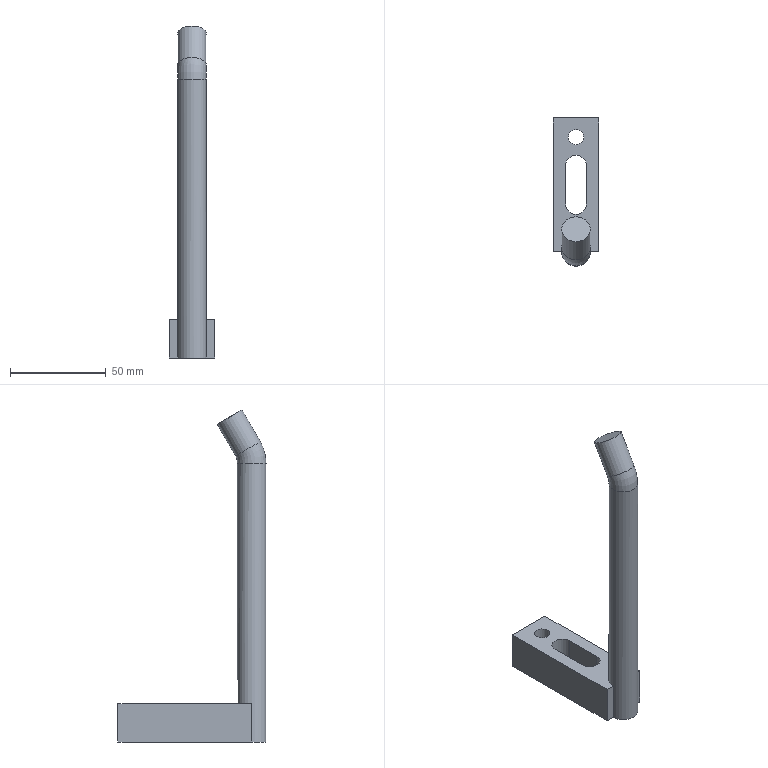Part | NX | features solid 2 | 1 solid | 16 faces | box 24 x 77.5 x 173.75 mm | volume 55083 mm3 | plane 10 | cylinder 5 | torus 1 | commonest cylinder face diameters 11 x2 15 x2 8 x1
STEP:
#1=CARTESIAN_POINT('',(-350.,-20.96,5.));
#2=VERTEX_POINT('',#1);
#3=CARTESIAN_POINT('',(-350.,-16.96,5.));
#4=DIRECTION('',(0.,0.,1.));
#5=DIRECTION('',(0.,-1.,0.));
#6=AXIS2_PLACEMENT_3D('',#3,#4,#5);
#7=CIRCLE('',#6,4.);
#8=EDGE_CURVE('',#2,#2,#7,.T.);
#9=ORIENTED_EDGE('',*,*,#8,.F.);
#10=EDGE_LOOP('',(#9));
#11=FACE_BOUND('',#10,.T.);
#12=CARTESIAN_POINT('',(-344.5,-51.96,5.));
#13=VERTEX_POINT('',#12);
#14=CARTESIAN_POINT('',(-344.5,-31.96,5.));
#15=VERTEX_POINT('',#14);
#16=CARTESIAN_POINT('',(-344.5,-41.96,5.));
#17=DIRECTION('',(0.,1.,0.));
#18=VECTOR('',#17,1000.);
#19=LINE('',#16,#18);
#20=EDGE_CURVE('',#13,#15,#19,.T.);
#21=ORIENTED_EDGE('',*,*,#20,.F.);
#22=CARTESIAN_POINT('',(-355.5,-51.96,5.));
#23=VERTEX_POINT('',#22);
#24=CARTESIAN_POINT('',(-350.,-51.96,5.));
#25=DIRECTION('',(0.,0.,-1.));
#26=DIRECTION('',(0.,1.,0.));
#27=AXIS2_PLACEMENT_3D('',#24,#25,#26);
#28=CIRCLE('',#27,5.5);
#29=EDGE_CURVE('',#13,#23,#28,.T.);
#30=ORIENTED_EDGE('',*,*,#29,.T.);
#31=CARTESIAN_POINT('',(-355.5,-31.96,5.));
#32=VERTEX_POINT('',#31);
#33=CARTESIAN_POINT('',(-355.5,-41.96,5.));
#34=DIRECTION('',(0.,1.,0.));
#35=VECTOR('',#34,1000.);
#36=LINE('',#33,#35);
#37=EDGE_CURVE('',#23,#32,#36,.T.);
#38=ORIENTED_EDGE('',*,*,#37,.T.);
#39=CARTESIAN_POINT('',(-350.,-31.96,5.));
#40=DIRECTION('',(0.,0.,-1.));
#41=DIRECTION('',(0.,1.,0.));
#42=AXIS2_PLACEMENT_3D('',#39,#40,#41);
#43=CIRCLE('',#42,5.5);
#44=EDGE_CURVE('',#32,#15,#43,.T.);
#45=ORIENTED_EDGE('',*,*,#44,.T.);
#46=EDGE_LOOP('',(#21,#30,#38,#45));
#47=FACE_BOUND('',#46,.T.);
#48=CARTESIAN_POINT('',(-357.5,-76.96,5.));
#49=VERTEX_POINT('',#48);
#50=CARTESIAN_POINT('',(-362.,-76.96,5.));
#51=VERTEX_POINT('',#50);
#52=CARTESIAN_POINT('',(-338.,-76.96,5.));
#53=DIRECTION('',(-1.,0.,0.));
#54=VECTOR('',#53,1000.);
#55=LINE('',#52,#54);
#56=EDGE_CURVE('',#49,#51,#55,.T.);
#57=ORIENTED_EDGE('',*,*,#56,.F.);
#58=CARTESIAN_POINT('',(-342.5,-76.96,5.));
#59=VERTEX_POINT('',#58);
#60=CARTESIAN_POINT('',(-350.,-76.96,5.));
#61=DIRECTION('',(0.,0.,1.));
#62=DIRECTION('',(1.,0.,0.));
#63=AXIS2_PLACEMENT_3D('',#60,#61,#62);
#64=CIRCLE('',#63,7.5);
#65=EDGE_CURVE('',#49,#59,#64,.F.);
#66=ORIENTED_EDGE('',*,*,#65,.T.);
#67=CARTESIAN_POINT('',(-338.,-76.96,5.));
#68=VERTEX_POINT('',#67);
#69=CARTESIAN_POINT('',(-338.,-76.96,5.));
#70=DIRECTION('',(-1.,0.,0.));
#71=VECTOR('',#70,1000.);
#72=LINE('',#69,#71);
#73=EDGE_CURVE('',#68,#59,#72,.T.);
#74=ORIENTED_EDGE('',*,*,#73,.F.);
#75=CARTESIAN_POINT('',(-338.,-6.96,5.));
#76=VERTEX_POINT('',#75);
#77=CARTESIAN_POINT('',(-338.,-6.96,5.));
#78=DIRECTION('',(0.,-1.,0.));
#79=VECTOR('',#78,1000.);
#80=LINE('',#77,#79);
#81=EDGE_CURVE('',#76,#68,#80,.T.);
#82=ORIENTED_EDGE('',*,*,#81,.F.);
#83=CARTESIAN_POINT('',(-362.,-6.96,5.));
#84=VERTEX_POINT('',#83);
#85=CARTESIAN_POINT('',(-362.,-6.96,5.));
#86=DIRECTION('',(1.,0.,0.));
#87=VECTOR('',#86,1000.);
#88=LINE('',#85,#87);
#89=EDGE_CURVE('',#84,#76,#88,.T.);
#90=ORIENTED_EDGE('',*,*,#89,.F.);
#91=CARTESIAN_POINT('',(-362.,-76.96,5.));
#92=DIRECTION('',(0.,1.,0.));
#93=VECTOR('',#92,1000.);
#94=LINE('',#91,#93);
#95=EDGE_CURVE('',#51,#84,#94,.T.);
#96=ORIENTED_EDGE('',*,*,#95,.F.);
#97=EDGE_LOOP('',(#57,#66,#74,#82,#90,#96));
#98=FACE_BOUND('',#97,.T.);
#99=CARTESIAN_POINT('',(-338.,-6.96,5.));
#100=DIRECTION('',(0.,0.,1.));
#101=DIRECTION('',(0.,1.,0.));
#102=AXIS2_PLACEMENT_3D('',#99,#100,#101);
#103=PLANE('',#102);
#104=ADVANCED_FACE('',(#11,#47,#98),#103,.T.);
#105=CARTESIAN_POINT('',(-357.5,-76.96,-15.));
#106=VERTEX_POINT('',#105);
#107=CARTESIAN_POINT('',(-362.,-76.96,-15.));
#108=VERTEX_POINT('',#107);
#109=CARTESIAN_POINT('',(-338.,-76.96,-15.));
#110=DIRECTION('',(-1.,0.,0.));
#111=VECTOR('',#110,1000.);
#112=LINE('',#109,#111);
#113=EDGE_CURVE('',#106,#108,#112,.T.);
#114=ORIENTED_EDGE('',*,*,#113,.T.);
#115=CARTESIAN_POINT('',(-362.,-6.96,-15.));
#116=VERTEX_POINT('',#115);
#117=CARTESIAN_POINT('',(-362.,-76.96,-15.));
#118=DIRECTION('',(0.,1.,0.));
#119=VECTOR('',#118,1000.);
#120=LINE('',#117,#119);
#121=EDGE_CURVE('',#108,#116,#120,.T.);
#122=ORIENTED_EDGE('',*,*,#121,.T.);
#123=CARTESIAN_POINT('',(-338.,-6.96,-15.));
#124=VERTEX_POINT('',#123);
#125=CARTESIAN_POINT('',(-362.,-6.96,-15.));
#126=DIRECTION('',(1.,0.,0.));
#127=VECTOR('',#126,1000.);
#128=LINE('',#125,#127);
#129=EDGE_CURVE('',#116,#124,#128,.T.);
#130=ORIENTED_EDGE('',*,*,#129,.T.);
#131=CARTESIAN_POINT('',(-338.,-76.96,-15.));
#132=VERTEX_POINT('',#131);
#133=CARTESIAN_POINT('',(-338.,-6.96,-15.));
#134=DIRECTION('',(0.,-1.,0.));
#135=VECTOR('',#134,1000.);
#136=LINE('',#133,#135);
#137=EDGE_CURVE('',#124,#132,#136,.T.);
#138=ORIENTED_EDGE('',*,*,#137,.T.);
#139=CARTESIAN_POINT('',(-342.5,-76.96,-15.));
#140=VERTEX_POINT('',#139);
#141=CARTESIAN_POINT('',(-338.,-76.96,-15.));
#142=DIRECTION('',(-1.,0.,0.));
#143=VECTOR('',#142,1000.);
#144=LINE('',#141,#143);
#145=EDGE_CURVE('',#132,#140,#144,.T.);
#146=ORIENTED_EDGE('',*,*,#145,.T.);
#147=CARTESIAN_POINT('',(-350.,-76.96,-15.));
#148=DIRECTION('',(0.,0.,-1.));
#149=DIRECTION('',(0.,1.,0.));
#150=AXIS2_PLACEMENT_3D('',#147,#148,#149);
#151=CIRCLE('',#150,7.5);
#152=EDGE_CURVE('',#140,#106,#151,.T.);
#153=ORIENTED_EDGE('',*,*,#152,.T.);
#154=EDGE_LOOP('',(#114,#122,#130,#138,#146,#153));
#155=FACE_BOUND('',#154,.T.);
#156=CARTESIAN_POINT('',(-355.5,-31.96,-15.));
#157=VERTEX_POINT('',#156);
#158=CARTESIAN_POINT('',(-344.5,-31.96,-15.));
#159=VERTEX_POINT('',#158);
#160=CARTESIAN_POINT('',(-350.,-31.96,-15.));
#161=DIRECTION('',(0.,0.,-1.));
#162=DIRECTION('',(0.,1.,0.));
#163=AXIS2_PLACEMENT_3D('',#160,#161,#162);
#164=CIRCLE('',#163,5.5);
#165=EDGE_CURVE('',#157,#159,#164,.T.);
#166=ORIENTED_EDGE('',*,*,#165,.F.);
#167=CARTESIAN_POINT('',(-355.5,-51.96,-15.));
#168=VERTEX_POINT('',#167);
#169=CARTESIAN_POINT('',(-355.5,-51.96,-15.));
#170=DIRECTION('',(0.,1.,0.));
#171=VECTOR('',#170,1000.);
#172=LINE('',#169,#171);
#173=EDGE_CURVE('',#168,#157,#172,.T.);
#174=ORIENTED_EDGE('',*,*,#173,.F.);
#175=CARTESIAN_POINT('',(-344.5,-51.96,-15.));
#176=VERTEX_POINT('',#175);
#177=CARTESIAN_POINT('',(-350.,-51.96,-15.));
#178=DIRECTION('',(0.,0.,-1.));
#179=DIRECTION('',(0.,1.,0.));
#180=AXIS2_PLACEMENT_3D('',#177,#178,#179);
#181=CIRCLE('',#180,5.5);
#182=EDGE_CURVE('',#176,#168,#181,.T.);
#183=ORIENTED_EDGE('',*,*,#182,.F.);
#184=CARTESIAN_POINT('',(-344.5,-51.96,-15.));
#185=DIRECTION('',(0.,1.,0.));
#186=VECTOR('',#185,1000.);
#187=LINE('',#184,#186);
#188=EDGE_CURVE('',#176,#159,#187,.T.);
#189=ORIENTED_EDGE('',*,*,#188,.T.);
#190=EDGE_LOOP('',(#166,#174,#183,#189));
#191=FACE_BOUND('',#190,.T.);
#192=CARTESIAN_POINT('',(-350.,-12.96,-15.));
#193=VERTEX_POINT('',#192);
#194=CARTESIAN_POINT('',(-350.,-16.96,-15.));
#195=DIRECTION('',(0.,0.,-1.));
#196=DIRECTION('',(0.,1.,0.));
#197=AXIS2_PLACEMENT_3D('',#194,#195,#196);
#198=CIRCLE('',#197,4.);
#199=EDGE_CURVE('',#193,#193,#198,.T.);
#200=ORIENTED_EDGE('',*,*,#199,.F.);
#201=EDGE_LOOP('',(#200));
#202=FACE_BOUND('',#201,.T.);
#203=CARTESIAN_POINT('',(-338.,-6.96,-15.));
#204=DIRECTION('',(0.,0.,1.));
#205=DIRECTION('',(0.,1.,0.));
#206=AXIS2_PLACEMENT_3D('',#203,#204,#205);
#207=PLANE('',#206);
#208=ADVANCED_FACE('',(#155,#191,#202),#207,.F.);
#209=ORIENTED_EDGE('',*,*,#137,.F.);
#210=CARTESIAN_POINT('',(-338.,-6.96,5.));
#211=DIRECTION('',(0.,0.,-1.));
#212=VECTOR('',#211,1000.);
#213=LINE('',#210,#212);
#214=EDGE_CURVE('',#76,#124,#213,.T.);
#215=ORIENTED_EDGE('',*,*,#214,.F.);
#216=ORIENTED_EDGE('',*,*,#81,.T.);
#217=CARTESIAN_POINT('',(-338.,-76.96,5.));
#218=DIRECTION('',(0.,0.,-1.));
#219=VECTOR('',#218,1000.);
#220=LINE('',#217,#219);
#221=EDGE_CURVE('',#68,#132,#220,.T.);
#222=ORIENTED_EDGE('',*,*,#221,.T.);
#223=EDGE_LOOP('',(#209,#215,#216,#222));
#224=FACE_BOUND('',#223,.T.);
#225=CARTESIAN_POINT('',(-338.,-6.96,5.));
#226=DIRECTION('',(-1.,0.,0.));
#227=DIRECTION('',(0.,1.,0.));
#228=AXIS2_PLACEMENT_3D('',#225,#226,#227);
#229=PLANE('',#228);
#230=ADVANCED_FACE('',(#224),#229,.F.);
#231=ORIENTED_EDGE('',*,*,#129,.F.);
#232=CARTESIAN_POINT('',(-362.,-6.96,5.));
#233=DIRECTION('',(0.,0.,-1.));
#234=VECTOR('',#233,1000.);
#235=LINE('',#232,#234);
#236=EDGE_CURVE('',#84,#116,#235,.T.);
#237=ORIENTED_EDGE('',*,*,#236,.F.);
#238=ORIENTED_EDGE('',*,*,#89,.T.);
#239=ORIENTED_EDGE('',*,*,#214,.T.);
#240=EDGE_LOOP('',(#231,#237,#238,#239));
#241=FACE_BOUND('',#240,.T.);
#242=CARTESIAN_POINT('',(-362.,-6.96,5.));
#243=DIRECTION('',(0.,-1.,0.));
#244=DIRECTION('',(0.,0.,1.));
#245=AXIS2_PLACEMENT_3D('',#242,#243,#244);
#246=PLANE('',#245);
#247=ADVANCED_FACE('',(#241),#246,.F.);
#248=ORIENTED_EDGE('',*,*,#121,.F.);
#249=CARTESIAN_POINT('',(-362.,-76.96,5.));
#250=DIRECTION('',(0.,0.,-1.));
#251=VECTOR('',#250,1000.);
#252=LINE('',#249,#251);
#253=EDGE_CURVE('',#51,#108,#252,.T.);
#254=ORIENTED_EDGE('',*,*,#253,.F.);
#255=ORIENTED_EDGE('',*,*,#95,.T.);
#256=ORIENTED_EDGE('',*,*,#236,.T.);
#257=EDGE_LOOP('',(#248,#254,#255,#256));
#258=FACE_BOUND('',#257,.T.);
#259=CARTESIAN_POINT('',(-362.,-76.96,5.));
#260=DIRECTION('',(1.,0.,0.));
#261=DIRECTION('',(0.,-1.,0.));
#262=AXIS2_PLACEMENT_3D('',#259,#260,#261);
#263=PLANE('',#262);
#264=ADVANCED_FACE('',(#258),#263,.F.);
#265=CARTESIAN_POINT('',(-357.5,-76.96,40.981));
#266=DIRECTION('',(0.,0.,-1.));
#267=VECTOR('',#266,1000.);
#268=LINE('',#265,#267);
#269=EDGE_CURVE('',#106,#49,#268,.F.);
#270=ORIENTED_EDGE('',*,*,#269,.T.);
#271=ORIENTED_EDGE('',*,*,#56,.T.);
#272=ORIENTED_EDGE('',*,*,#253,.T.);
#273=ORIENTED_EDGE('',*,*,#113,.F.);
#274=EDGE_LOOP('',(#270,#271,#272,#273));
#275=FACE_BOUND('',#274,.T.);
#276=CARTESIAN_POINT('',(-338.,-76.96,5.));
#277=DIRECTION('',(0.,1.,0.));
#278=DIRECTION('',(0.,0.,-1.));
#279=AXIS2_PLACEMENT_3D('',#276,#277,#278);
#280=PLANE('',#279);
#281=ADVANCED_FACE('',(#275),#280,.F.);
#282=ORIENTED_EDGE('',*,*,#65,.F.);
#283=ORIENTED_EDGE('',*,*,#269,.F.);
#284=ORIENTED_EDGE('',*,*,#152,.F.);
#285=CARTESIAN_POINT('',(-342.5,-76.96,40.981));
#286=DIRECTION('',(0.,0.,-1.));
#287=VECTOR('',#286,1000.);
#288=LINE('',#285,#287);
#289=EDGE_CURVE('',#59,#140,#288,.T.);
#290=ORIENTED_EDGE('',*,*,#289,.F.);
#291=EDGE_LOOP('',(#282,#283,#284,#290));
#292=FACE_BOUND('',#291,.T.);
#293=CARTESIAN_POINT('',(-350.,-69.46,130.981));
#294=VERTEX_POINT('',#293);
#295=CARTESIAN_POINT('',(-350.,-76.96,130.981));
#296=DIRECTION('',(0.,0.,-1.));
#297=DIRECTION('',(0.,1.,0.));
#298=AXIS2_PLACEMENT_3D('',#295,#296,#297);
#299=CIRCLE('',#298,7.5);
#300=EDGE_CURVE('',#294,#294,#299,.T.);
#301=ORIENTED_EDGE('',*,*,#300,.T.);
#302=EDGE_LOOP('',(#301));
#303=FACE_BOUND('',#302,.T.);
#304=CARTESIAN_POINT('',(-350.,-76.96,40.981));
#305=DIRECTION('',(0.,0.,-1.));
#306=DIRECTION('',(0.,-1.,0.));
#307=AXIS2_PLACEMENT_3D('',#304,#305,#306);
#308=CYLINDRICAL_SURFACE('',#307,7.5);
#309=ADVANCED_FACE('',(#292,#303),#308,.T.);
#310=ORIENTED_EDGE('',*,*,#289,.T.);
#311=ORIENTED_EDGE('',*,*,#145,.F.);
#312=ORIENTED_EDGE('',*,*,#221,.F.);
#313=ORIENTED_EDGE('',*,*,#73,.T.);
#314=EDGE_LOOP('',(#310,#311,#312,#313));
#315=FACE_BOUND('',#314,.T.);
#316=CARTESIAN_POINT('',(-338.,-76.96,5.));
#317=DIRECTION('',(0.,1.,0.));
#318=DIRECTION('',(0.,0.,-1.));
#319=AXIS2_PLACEMENT_3D('',#316,#317,#318);
#320=PLANE('',#319);
#321=ADVANCED_FACE('',(#315),#320,.F.);
#322=ORIENTED_EDGE('',*,*,#8,.T.);
#323=EDGE_LOOP('',(#322));
#324=FACE_BOUND('',#323,.T.);
#325=ORIENTED_EDGE('',*,*,#199,.T.);
#326=EDGE_LOOP('',(#325));
#327=FACE_BOUND('',#326,.T.);
#328=CARTESIAN_POINT('',(-350.,-16.96,5.));
#329=DIRECTION('',(0.,0.,-1.));
#330=DIRECTION('',(0.,-1.,0.));
#331=AXIS2_PLACEMENT_3D('',#328,#329,#330);
#332=CYLINDRICAL_SURFACE('',#331,4.);
#333=ADVANCED_FACE('',(#324,#327),#332,.F.);
#334=ORIENTED_EDGE('',*,*,#29,.F.);
#335=CARTESIAN_POINT('',(-344.5,-51.96,5.));
#336=DIRECTION('',(0.,0.,1.));
#337=VECTOR('',#336,1000.);
#338=LINE('',#335,#337);
#339=EDGE_CURVE('',#176,#13,#338,.T.);
#340=ORIENTED_EDGE('',*,*,#339,.F.);
#341=ORIENTED_EDGE('',*,*,#182,.T.);
#342=CARTESIAN_POINT('',(-355.5,-51.96,5.));
#343=DIRECTION('',(0.,0.,1.));
#344=VECTOR('',#343,1000.);
#345=LINE('',#342,#344);
#346=EDGE_CURVE('',#168,#23,#345,.T.);
#347=ORIENTED_EDGE('',*,*,#346,.T.);
#348=EDGE_LOOP('',(#334,#340,#341,#347));
#349=FACE_BOUND('',#348,.T.);
#350=CARTESIAN_POINT('',(-350.,-51.96,5.));
#351=DIRECTION('',(0.,0.,1.));
#352=DIRECTION('',(0.,1.,0.));
#353=AXIS2_PLACEMENT_3D('',#350,#351,#352);
#354=CYLINDRICAL_SURFACE('',#353,5.5);
#355=ADVANCED_FACE('',(#349),#354,.F.);
#356=ORIENTED_EDGE('',*,*,#37,.F.);
#357=ORIENTED_EDGE('',*,*,#346,.F.);
#358=ORIENTED_EDGE('',*,*,#173,.T.);
#359=CARTESIAN_POINT('',(-355.5,-31.96,5.));
#360=DIRECTION('',(0.,0.,1.));
#361=VECTOR('',#360,1000.);
#362=LINE('',#359,#361);
#363=EDGE_CURVE('',#157,#32,#362,.T.);
#364=ORIENTED_EDGE('',*,*,#363,.T.);
#365=EDGE_LOOP('',(#356,#357,#358,#364));
#366=FACE_BOUND('',#365,.T.);
#367=CARTESIAN_POINT('',(-355.5,-41.96,5.));
#368=DIRECTION('',(-1.,0.,0.));
#369=DIRECTION('',(0.,0.,-1.));
#370=AXIS2_PLACEMENT_3D('',#367,#368,#369);
#371=PLANE('',#370);
#372=ADVANCED_FACE('',(#366),#371,.F.);
#373=ORIENTED_EDGE('',*,*,#44,.F.);
#374=ORIENTED_EDGE('',*,*,#363,.F.);
#375=ORIENTED_EDGE('',*,*,#165,.T.);
#376=CARTESIAN_POINT('',(-344.5,-31.96,5.));
#377=DIRECTION('',(0.,0.,1.));
#378=VECTOR('',#377,1000.);
#379=LINE('',#376,#378);
#380=EDGE_CURVE('',#159,#15,#379,.T.);
#381=ORIENTED_EDGE('',*,*,#380,.T.);
#382=EDGE_LOOP('',(#373,#374,#375,#381));
#383=FACE_BOUND('',#382,.T.);
#384=CARTESIAN_POINT('',(-350.,-31.96,5.));
#385=DIRECTION('',(0.,0.,1.));
#386=DIRECTION('',(0.,1.,0.));
#387=AXIS2_PLACEMENT_3D('',#384,#385,#386);
#388=CYLINDRICAL_SURFACE('',#387,5.5);
#389=ADVANCED_FACE('',(#383),#388,.F.);
#390=ORIENTED_EDGE('',*,*,#20,.T.);
#391=ORIENTED_EDGE('',*,*,#380,.F.);
#392=ORIENTED_EDGE('',*,*,#188,.F.);
#393=ORIENTED_EDGE('',*,*,#339,.T.);
#394=EDGE_LOOP('',(#390,#391,#392,#393));
#395=FACE_BOUND('',#394,.T.);
#396=CARTESIAN_POINT('',(-344.5,-41.96,5.));
#397=DIRECTION('',(1.,0.,0.));
#398=DIRECTION('',(0.,0.,1.));
#399=AXIS2_PLACEMENT_3D('',#396,#397,#398);
#400=PLANE('',#399);
#401=ADVANCED_FACE('',(#395),#400,.F.);
#402=CARTESIAN_POINT('',(-350.,-68.455,134.731));
#403=VERTEX_POINT('',#402);
#404=CARTESIAN_POINT('',(-350.,-74.951,138.481));
#405=DIRECTION('',(0.,-0.5,-0.866));
#406=DIRECTION('',(0.,0.866,-0.5));
#407=AXIS2_PLACEMENT_3D('',#404,#405,#406);
#408=CIRCLE('',#407,7.5);
#409=EDGE_CURVE('',#403,#403,#408,.T.);
#410=ORIENTED_EDGE('',*,*,#409,.F.);
#411=EDGE_LOOP('',(#410));
#412=FACE_BOUND('',#411,.T.);
#413=CARTESIAN_POINT('',(-350.,-58.918,151.25));
#414=VERTEX_POINT('',#413);
#415=CARTESIAN_POINT('',(-350.,-65.413,155.));
#416=DIRECTION('',(0.,-0.5,-0.866));
#417=DIRECTION('',(0.,0.866,-0.5));
#418=AXIS2_PLACEMENT_3D('',#415,#416,#417);
#419=CIRCLE('',#418,7.5);
#420=EDGE_CURVE('',#414,#414,#419,.T.);
#421=ORIENTED_EDGE('',*,*,#420,.T.);
#422=EDGE_LOOP('',(#421));
#423=FACE_BOUND('',#422,.T.);
#424=CARTESIAN_POINT('',(-350.,-74.951,138.481));
#425=DIRECTION('',(0.,0.5,0.866));
#426=DIRECTION('',(0.,0.866,-0.5));
#427=AXIS2_PLACEMENT_3D('',#424,#425,#426);
#428=CYLINDRICAL_SURFACE('',#427,7.5);
#429=ADVANCED_FACE('',(#412,#423),#428,.T.);
#430=ORIENTED_EDGE('',*,*,#300,.F.);
#431=EDGE_LOOP('',(#430));
#432=FACE_BOUND('',#431,.T.);
#433=ORIENTED_EDGE('',*,*,#409,.T.);
#434=EDGE_LOOP('',(#433));
#435=FACE_BOUND('',#434,.T.);
#436=CARTESIAN_POINT('',(-350.,-61.96,130.981));
#437=DIRECTION('',(1.,0.,0.));
#438=DIRECTION('',(0.,0.,1.));
#439=AXIS2_PLACEMENT_3D('',#436,#437,#438);
#440=TOROIDAL_SURFACE('',#439,15.,7.5);
#441=ADVANCED_FACE('',(#432,#435),#440,.T.);
#442=ORIENTED_EDGE('',*,*,#420,.F.);
#443=EDGE_LOOP('',(#442));
#444=FACE_BOUND('',#443,.T.);
#445=CARTESIAN_POINT('',(-350.,-65.413,155.));
#446=DIRECTION('',(0.,0.5,0.866));
#447=DIRECTION('',(0.,0.866,-0.5));
#448=AXIS2_PLACEMENT_3D('',#445,#446,#447);
#449=PLANE('',#448);
#450=ADVANCED_FACE('',(#444),#449,.T.);
#451=CLOSED_SHELL('',(#104,#208,#230,#247,#264,#281,#309,#321,#333,#355,#372,#389,#401,#429,#441,#450));
#452=MANIFOLD_SOLID_BREP('',#451);
#453=(LENGTH_UNIT()NAMED_UNIT(*)SI_UNIT(.MILLI.,.METRE.));
#454=UNCERTAINTY_MEASURE_WITH_UNIT(LENGTH_MEASURE(0.00001),#453,'','');
#455=(NAMED_UNIT(*)PLANE_ANGLE_UNIT()SI_UNIT($,.RADIAN.));
#456=(NAMED_UNIT(*)SI_UNIT($,.STERADIAN.)SOLID_ANGLE_UNIT());
#457=(GEOMETRIC_REPRESENTATION_CONTEXT(3)GLOBAL_UNCERTAINTY_ASSIGNED_CONTEXT((#454))GLOBAL_UNIT_ASSIGNED_CONTEXT((#453,#455,#456))REPRESENTATION_CONTEXT('',''));
#458=ADVANCED_BREP_SHAPE_REPRESENTATION('',(#452),#457);